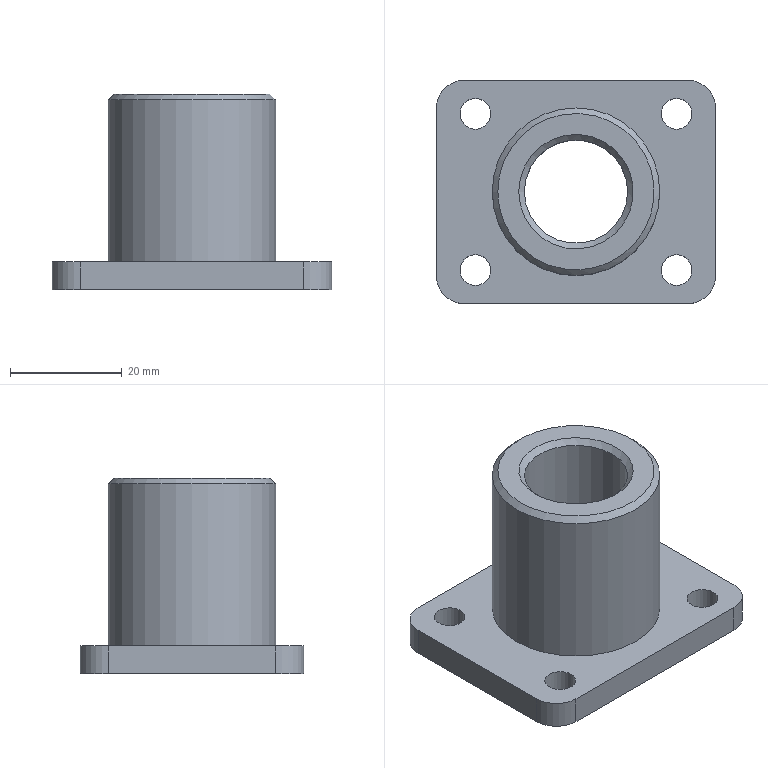CAM job | NX | 3-axis milling, drilling | part box 50 x 40 x 35 mm | stock box 60 x 50 x 40 mm
Tools:
number,name,description,diameter,corner_radius,flute_length,length,flutes
1,D50面刀,,50.0,0.0,50.0,75.0,2
4,D10倒角刀,,10.0,0.0,50.0,75.0,2
6,14钻头,,14.0,0.0,50.0,75.0,2
2,D14开粗,,14.0,0.0,50.0,75.0,2
5,5.5钻头,,5.5,0.0,50.0,75.0,2
7,D12-1.5,,18.0,0.0,1.0,80.0,2
3,D16精光,,16.0,0.0,50.0,75.0,2
Operations:
program,operation,operation_type,tool,method,geometry_group,spindle_rpm,surface_speed,feed_per_tooth,feed_cut,feed_plunge,cut_length_mm,path_length_mm,cut_time_min,machine_time_min
G54,PLANAR_MILL,PlanarMilling,D50面刀,METHOD,WORKPIECE,3500.0,549.0,0.1143,800.0,100.0,146.0,180.0,0.1825,0.1859
G54,DRILLING,Operation,D10倒角刀,METHOD,WORKPIECE,1600.0,50.0,0.0625,200.0,0.0,5.0,50.0,0.025,0.0295
G54,DRILLING_COPY,Operation,14钻头,METHOD,WORKPIECE,1600.0,70.0,0.0781,250.0,0.0,48.0,136.0,0.192,0.2008
G54,ADAPTIVE_MILLING,CavityMilling,D14开粗,METHOD,WORKPIECE,6500.0,285.0,0.1538,2000.0,100.0,4467.235,4692.328,2.23,2.252
G54,HOLE_MILLING,CylinderMilling,D14开粗,METHOD,WORKPIECE,3500.0,153.0,0.0714,500.0,100.0,588.105,664.105,1.176,1.184
G54,PLANAR_MILL_2,PlanarMilling,D14开粗,METHOD,WORKPIECE,3500.0,153.0,0.0429,300.0,100.0,22.279,130.279,0.0743,0.0851
G54,DRILLING_1,Operation,D10倒角刀,METHOD,WORKPIECE,1600.0,50.0,0.0781,250.0,0.0,23.0,255.41,0.092,0.1152
G54,PLANAR_MILL_1,PlanarMilling,D10倒角刀,METHOD,WORKPIECE,3500.0,109.0,0.1429,1000.0,100.0,117.097,159.097,0.1171,0.1213
G54,PLANAR_MILL_1_COPY,PlanarMilling,D10倒角刀,METHOD,WORKPIECE,3500.0,109.0,0.1429,1000.0,100.0,57.853,99.853,0.0579,0.0621
G54,PLANAR_MILL_1_COPY_COPY,PlanarMilling,D10倒角刀,METHOD,WORKPIECE,3500.0,109.0,0.1429,1000.0,100.0,193.637,293.637,0.1936,0.2036
G54,DRILLING_1_COPY,Operation,5.5钻头,METHOD,WORKPIECE,2000.0,34.0,0.0375,150.0,0.0,44.0,297.41,0.2933,0.3187
G54,THREAD_MILLING,ThreadMilling,D12-1.5,METHOD,WORKPIECE,2000.0,87.0,0.05,200.0,100.0,124.89,201.89,0.6245,0.6322
G54,PLANAR_MILL_3,PlanarMilling,D16精光,METHOD,WORKPIECE,3500.0,175.0,0.0857,600.0,100.0,231.965,339.965,0.3866,0.3974
G54,PLANAR_MILL_3_COPY,PlanarMilling,D16精光,METHOD,WORKPIECE,3500.0,175.0,0.0857,600.0,100.0,332.371,428.371,0.554,0.5636
G54,PLANAR_MILL_3_COPY_COPY,PlanarMilling,D16精光,METHOD,WORKPIECE,3500.0,175.0,0.0857,600.0,100.0,156.796,252.786,0.2613,0.2709
G55,PLANAR_MILL_COPY,PlanarMilling,D50面刀,METHOD,G55,3500.0,549.0,0.1143,800.0,100.0,146.0,180.0,0.1825,0.1859
G55,PLANAR_MILL_4,PlanarMilling,D10倒角刀,METHOD,G55,3500.0,109.0,0.1143,800.0,100.0,191.124,230.124,0.2389,0.2428
G55,PLANAR_MILL_4_COPY,PlanarMilling,D10倒角刀,METHOD,G55,3500.0,109.0,0.1143,800.0,100.0,57.853,99.853,0.0723,0.0765
G55,DRILLING_2,Operation,D10倒角刀,METHOD,G55,2000.0,62.0,0.0625,250.0,0.0,23.0,195.41,0.092,0.1092